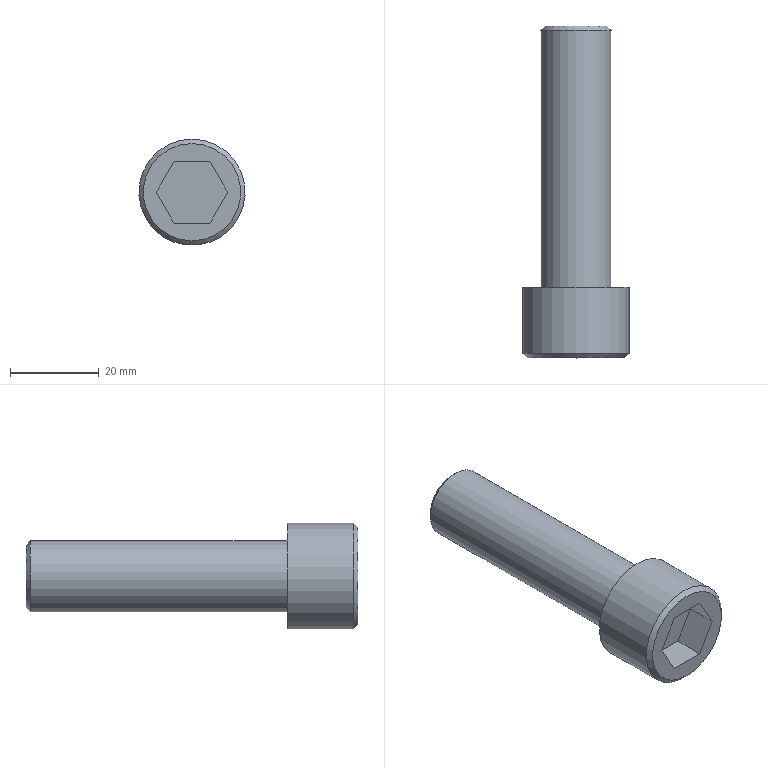Part | STEP file | solid 170 | 1 solid | 14 faces | box 24 x 75 x 24 mm | volume 17852 mm3 | plane 10 | cylinder 2 | cone 2 | commonest cylinder face diameters 16 x1 24 x1